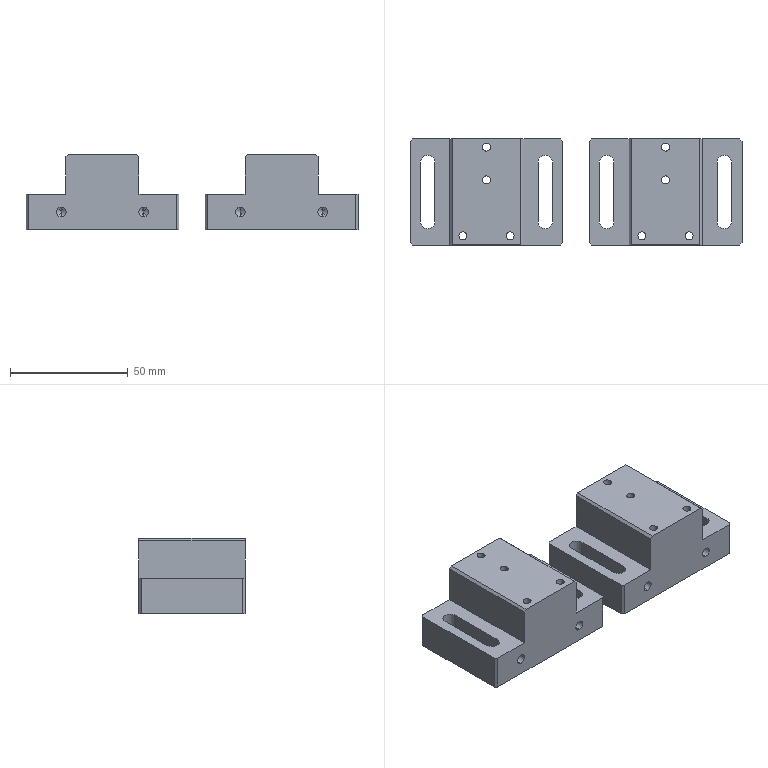NC program | NX | posted with a generic post | part box 140.92 x 45 x 32 mm
Lines 1 to 34 of 10208:
N10 G17 G21 G94 G90
(FLOOR_WALL_COPY , TOOL : D80)
N12 T19 M6
N14 G54
N16 G17 G0 G90 X183.92 Y22.5 S6500 M3
N18 G43 Z30. H19
N20 Z5.
N22 G94 G1 Z2. F1500.
N24 X180.92
N26 X-40.
N28 X-43.
N30 Z5.
N32 G0 Z30.
N34 X183.92
N36 Z4.
N38 G1 Z1.
N40 X180.92
N42 X-40.
N44 X-43.
N46 Z4.
N48 G0 Z30.
N50 X183.92
N52 Z3.
N54 G1 Z0.
N56 X180.92
N58 X-40.
N60 X-43.
N62 Z3.
N64 G0 Z30.
N66 M5